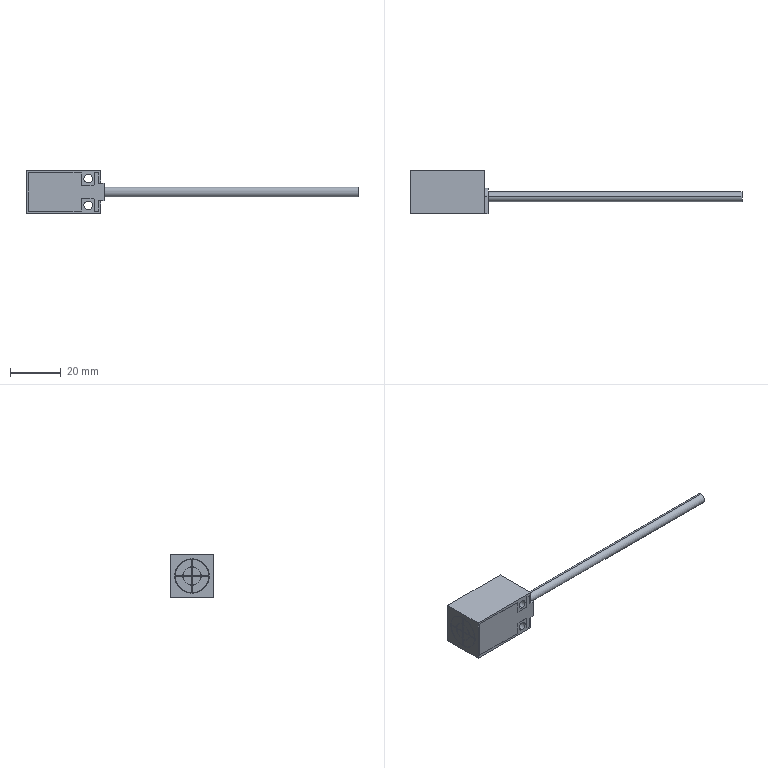Part | 1 solid | 91 faces | box 130.8 x 17 x 17 mm | volume 9325 mm3 | plane 62 | cylinder 29 | commonest cylinder face diameters 3.4 x6 1 x4 6.9 x4 7.3 x4 13.1 x4 0.4 x2